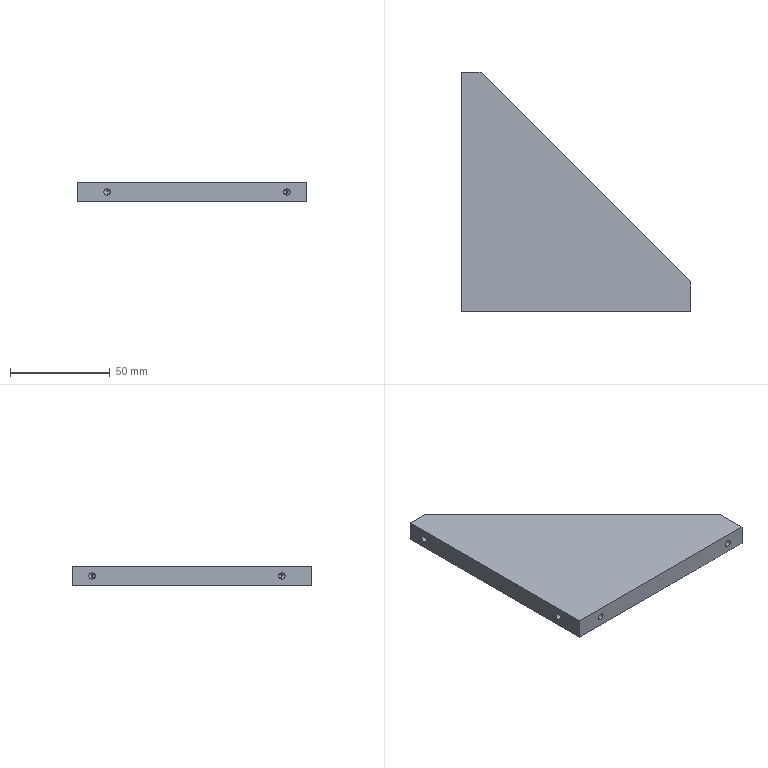Part | SolidWorks | features HoleWzd 4, ICE 4, Fillet 2, ExtruThin 1, Gusset 1 | 1 solid | 23 faces | box 115 x 120 x 10 mm | volume 82518 mm3 | cylinder 8 | cone 8 | plane 7 | commonest cylinder face diameters 3.3 x8
STEP:
#1=CARTESIAN_POINT('',(10.1,110.,28.35));
#2=VERTEX_POINT('',#1);
#3=CARTESIAN_POINT('',(10.1,110.,31.65));
#4=VERTEX_POINT('',#3);
#5=CARTESIAN_POINT('',(10.1,110.,30.));
#6=DIRECTION('',(-1.,0.,0.));
#7=DIRECTION('',(0.,0.,1.));
#8=AXIS2_PLACEMENT_3D('',#5,#6,#7);
#9=CIRCLE('',#8,1.65);
#10=EDGE_CURVE('',#2,#4,#9,.T.);
#11=ORIENTED_EDGE('',*,*,#10,.F.);
#12=CARTESIAN_POINT('',(0.,110.,28.35));
#13=VERTEX_POINT('',#12);
#14=CARTESIAN_POINT('',(0.,110.,28.35));
#15=DIRECTION('',(-1.,0.,0.));
#16=VECTOR('',#15,1000.);
#17=LINE('',#14,#16);
#18=EDGE_CURVE('',#2,#13,#17,.T.);
#19=ORIENTED_EDGE('',*,*,#18,.T.);
#20=CARTESIAN_POINT('',(0.,110.,31.65));
#21=VERTEX_POINT('',#20);
#22=CARTESIAN_POINT('',(0.,110.,30.));
#23=DIRECTION('',(-1.,0.,0.));
#24=DIRECTION('',(0.,0.,1.));
#25=AXIS2_PLACEMENT_3D('',#22,#23,#24);
#26=CIRCLE('',#25,1.65);
#27=EDGE_CURVE('',#13,#21,#26,.T.);
#28=ORIENTED_EDGE('',*,*,#27,.T.);
#29=CARTESIAN_POINT('',(0.,110.,31.65));
#30=DIRECTION('',(-1.,0.,0.));
#31=VECTOR('',#30,1000.);
#32=LINE('',#29,#31);
#33=EDGE_CURVE('',#4,#21,#32,.T.);
#34=ORIENTED_EDGE('',*,*,#33,.F.);
#35=EDGE_LOOP('',(#11,#19,#28,#34));
#36=FACE_OUTER_BOUND('',#35,.T.);
#37=CARTESIAN_POINT('',(0.,110.,30.));
#38=DIRECTION('',(-1.,0.,0.));
#39=DIRECTION('',(0.,0.,1.));
#40=AXIS2_PLACEMENT_3D('',#37,#38,#39);
#41=CYLINDRICAL_SURFACE('',#40,1.65);
#42=ADVANCED_FACE('',(#36),#41,.F.);
#43=CARTESIAN_POINT('',(11.091,110.,30.));
#44=VERTEX_POINT('',#43);
#45=CARTESIAN_POINT('',(10.1,110.,31.65));
#46=DIRECTION('',(-0.515,0.,0.8572));
#47=VECTOR('',#46,1000.);
#48=LINE('',#45,#47);
#49=EDGE_CURVE('',#44,#4,#48,.T.);
#50=ORIENTED_EDGE('',*,*,#49,.F.);
#51=CARTESIAN_POINT('',(10.1,110.,28.35));
#52=DIRECTION('',(-0.515,0.,-0.8572));
#53=VECTOR('',#52,1000.);
#54=LINE('',#51,#53);
#55=EDGE_CURVE('',#44,#2,#54,.T.);
#56=ORIENTED_EDGE('',*,*,#55,.T.);
#57=ORIENTED_EDGE('',*,*,#10,.T.);
#58=EDGE_LOOP('',(#50,#56,#57));
#59=FACE_OUTER_BOUND('',#58,.T.);
#60=CARTESIAN_POINT('',(10.1,110.,30.));
#61=DIRECTION('',(-1.,0.,0.));
#62=DIRECTION('',(0.,0.,1.));
#63=AXIS2_PLACEMENT_3D('',#60,#61,#62);
#64=CONICAL_SURFACE('',#63,1.65,1.03);
#65=ADVANCED_FACE('',(#59),#64,.F.);
#66=CARTESIAN_POINT('',(10.1,15.,28.35));
#67=VERTEX_POINT('',#66);
#68=CARTESIAN_POINT('',(10.1,15.,31.65));
#69=VERTEX_POINT('',#68);
#70=CARTESIAN_POINT('',(10.1,15.,30.));
#71=DIRECTION('',(-1.,0.,0.));
#72=DIRECTION('',(0.,0.,1.));
#73=AXIS2_PLACEMENT_3D('',#70,#71,#72);
#74=CIRCLE('',#73,1.65);
#75=EDGE_CURVE('',#67,#69,#74,.T.);
#76=ORIENTED_EDGE('',*,*,#75,.F.);
#77=CARTESIAN_POINT('',(0.,15.,28.35));
#78=VERTEX_POINT('',#77);
#79=CARTESIAN_POINT('',(0.,15.,28.35));
#80=DIRECTION('',(-1.,0.,0.));
#81=VECTOR('',#80,1000.);
#82=LINE('',#79,#81);
#83=EDGE_CURVE('',#67,#78,#82,.T.);
#84=ORIENTED_EDGE('',*,*,#83,.T.);
#85=CARTESIAN_POINT('',(0.,15.,31.65));
#86=VERTEX_POINT('',#85);
#87=CARTESIAN_POINT('',(0.,15.,30.));
#88=DIRECTION('',(-1.,0.,0.));
#89=DIRECTION('',(0.,0.,1.));
#90=AXIS2_PLACEMENT_3D('',#87,#88,#89);
#91=CIRCLE('',#90,1.65);
#92=EDGE_CURVE('',#78,#86,#91,.T.);
#93=ORIENTED_EDGE('',*,*,#92,.T.);
#94=CARTESIAN_POINT('',(0.,15.,31.65));
#95=DIRECTION('',(-1.,0.,0.));
#96=VECTOR('',#95,1000.);
#97=LINE('',#94,#96);
#98=EDGE_CURVE('',#69,#86,#97,.T.);
#99=ORIENTED_EDGE('',*,*,#98,.F.);
#100=EDGE_LOOP('',(#76,#84,#93,#99));
#101=FACE_OUTER_BOUND('',#100,.T.);
#102=CARTESIAN_POINT('',(0.,15.,30.));
#103=DIRECTION('',(-1.,0.,0.));
#104=DIRECTION('',(0.,0.,1.));
#105=AXIS2_PLACEMENT_3D('',#102,#103,#104);
#106=CYLINDRICAL_SURFACE('',#105,1.65);
#107=ADVANCED_FACE('',(#101),#106,.F.);
#108=CARTESIAN_POINT('',(11.091,15.,30.));
#109=VERTEX_POINT('',#108);
#110=CARTESIAN_POINT('',(10.1,15.,31.65));
#111=DIRECTION('',(-0.515,0.,0.8572));
#112=VECTOR('',#111,1000.);
#113=LINE('',#110,#112);
#114=EDGE_CURVE('',#109,#69,#113,.T.);
#115=ORIENTED_EDGE('',*,*,#114,.F.);
#116=CARTESIAN_POINT('',(10.1,15.,28.35));
#117=DIRECTION('',(-0.515,0.,-0.8572));
#118=VECTOR('',#117,1000.);
#119=LINE('',#116,#118);
#120=EDGE_CURVE('',#109,#67,#119,.T.);
#121=ORIENTED_EDGE('',*,*,#120,.T.);
#122=ORIENTED_EDGE('',*,*,#75,.T.);
#123=EDGE_LOOP('',(#115,#121,#122));
#124=FACE_OUTER_BOUND('',#123,.T.);
#125=CARTESIAN_POINT('',(10.1,15.,30.));
#126=DIRECTION('',(-1.,0.,0.));
#127=DIRECTION('',(0.,0.,1.));
#128=AXIS2_PLACEMENT_3D('',#125,#126,#127);
#129=CONICAL_SURFACE('',#128,1.65,1.03);
#130=ADVANCED_FACE('',(#124),#129,.F.);
#131=CARTESIAN_POINT('',(105.,10.1,31.65));
#132=VERTEX_POINT('',#131);
#133=CARTESIAN_POINT('',(105.,10.1,28.35));
#134=VERTEX_POINT('',#133);
#135=CARTESIAN_POINT('',(105.,10.1,30.));
#136=DIRECTION('',(0.,-1.,0.));
#137=DIRECTION('',(0.,0.,-1.));
#138=AXIS2_PLACEMENT_3D('',#135,#136,#137);
#139=CIRCLE('',#138,1.65);
#140=EDGE_CURVE('',#132,#134,#139,.T.);
#141=ORIENTED_EDGE('',*,*,#140,.F.);
#142=CARTESIAN_POINT('',(105.,0.,31.65));
#143=VERTEX_POINT('',#142);
#144=CARTESIAN_POINT('',(105.,0.,31.65));
#145=DIRECTION('',(0.,-1.,0.));
#146=VECTOR('',#145,1000.);
#147=LINE('',#144,#146);
#148=EDGE_CURVE('',#132,#143,#147,.T.);
#149=ORIENTED_EDGE('',*,*,#148,.T.);
#150=CARTESIAN_POINT('',(105.,0.,28.35));
#151=VERTEX_POINT('',#150);
#152=CARTESIAN_POINT('',(105.,0.,30.));
#153=DIRECTION('',(0.,-1.,0.));
#154=DIRECTION('',(0.,0.,-1.));
#155=AXIS2_PLACEMENT_3D('',#152,#153,#154);
#156=CIRCLE('',#155,1.65);
#157=EDGE_CURVE('',#143,#151,#156,.T.);
#158=ORIENTED_EDGE('',*,*,#157,.T.);
#159=CARTESIAN_POINT('',(105.,0.,28.35));
#160=DIRECTION('',(0.,-1.,0.));
#161=VECTOR('',#160,1000.);
#162=LINE('',#159,#161);
#163=EDGE_CURVE('',#134,#151,#162,.T.);
#164=ORIENTED_EDGE('',*,*,#163,.F.);
#165=EDGE_LOOP('',(#141,#149,#158,#164));
#166=FACE_OUTER_BOUND('',#165,.T.);
#167=CARTESIAN_POINT('',(105.,0.,30.));
#168=DIRECTION('',(0.,-1.,0.));
#169=DIRECTION('',(0.,0.,-1.));
#170=AXIS2_PLACEMENT_3D('',#167,#168,#169);
#171=CYLINDRICAL_SURFACE('',#170,1.65);
#172=ADVANCED_FACE('',(#166),#171,.F.);
#173=CARTESIAN_POINT('',(105.,11.091,30.));
#174=VERTEX_POINT('',#173);
#175=CARTESIAN_POINT('',(105.,10.1,28.35));
#176=DIRECTION('',(0.,-0.515,-0.8572));
#177=VECTOR('',#176,1000.);
#178=LINE('',#175,#177);
#179=EDGE_CURVE('',#174,#134,#178,.T.);
#180=ORIENTED_EDGE('',*,*,#179,.F.);
#181=CARTESIAN_POINT('',(105.,10.1,31.65));
#182=DIRECTION('',(0.,-0.515,0.8572));
#183=VECTOR('',#182,1000.);
#184=LINE('',#181,#183);
#185=EDGE_CURVE('',#174,#132,#184,.T.);
#186=ORIENTED_EDGE('',*,*,#185,.T.);
#187=ORIENTED_EDGE('',*,*,#140,.T.);
#188=EDGE_LOOP('',(#180,#186,#187));
#189=FACE_OUTER_BOUND('',#188,.T.);
#190=CARTESIAN_POINT('',(105.,10.1,30.));
#191=DIRECTION('',(0.,-1.,0.));
#192=DIRECTION('',(0.,0.,-1.));
#193=AXIS2_PLACEMENT_3D('',#190,#191,#192);
#194=CONICAL_SURFACE('',#193,1.65,1.03);
#195=ADVANCED_FACE('',(#189),#194,.F.);
#196=CARTESIAN_POINT('',(15.,10.1,31.65));
#197=VERTEX_POINT('',#196);
#198=CARTESIAN_POINT('',(15.,10.1,28.35));
#199=VERTEX_POINT('',#198);
#200=CARTESIAN_POINT('',(15.,10.1,30.));
#201=DIRECTION('',(0.,-1.,0.));
#202=DIRECTION('',(0.,0.,-1.));
#203=AXIS2_PLACEMENT_3D('',#200,#201,#202);
#204=CIRCLE('',#203,1.65);
#205=EDGE_CURVE('',#197,#199,#204,.T.);
#206=ORIENTED_EDGE('',*,*,#205,.F.);
#207=CARTESIAN_POINT('',(15.,0.,31.65));
#208=VERTEX_POINT('',#207);
#209=CARTESIAN_POINT('',(15.,0.,31.65));
#210=DIRECTION('',(0.,-1.,0.));
#211=VECTOR('',#210,1000.);
#212=LINE('',#209,#211);
#213=EDGE_CURVE('',#197,#208,#212,.T.);
#214=ORIENTED_EDGE('',*,*,#213,.T.);
#215=CARTESIAN_POINT('',(15.,0.,28.35));
#216=VERTEX_POINT('',#215);
#217=CARTESIAN_POINT('',(15.,0.,30.));
#218=DIRECTION('',(0.,-1.,0.));
#219=DIRECTION('',(0.,0.,-1.));
#220=AXIS2_PLACEMENT_3D('',#217,#218,#219);
#221=CIRCLE('',#220,1.65);
#222=EDGE_CURVE('',#208,#216,#221,.T.);
#223=ORIENTED_EDGE('',*,*,#222,.T.);
#224=CARTESIAN_POINT('',(15.,0.,28.35));
#225=DIRECTION('',(0.,-1.,0.));
#226=VECTOR('',#225,1000.);
#227=LINE('',#224,#226);
#228=EDGE_CURVE('',#199,#216,#227,.T.);
#229=ORIENTED_EDGE('',*,*,#228,.F.);
#230=EDGE_LOOP('',(#206,#214,#223,#229));
#231=FACE_OUTER_BOUND('',#230,.T.);
#232=CARTESIAN_POINT('',(15.,0.,30.));
#233=DIRECTION('',(0.,-1.,0.));
#234=DIRECTION('',(0.,0.,-1.));
#235=AXIS2_PLACEMENT_3D('',#232,#233,#234);
#236=CYLINDRICAL_SURFACE('',#235,1.65);
#237=ADVANCED_FACE('',(#231),#236,.F.);
#238=CARTESIAN_POINT('',(15.,11.091,30.));
#239=VERTEX_POINT('',#238);
#240=CARTESIAN_POINT('',(15.,10.1,28.35));
#241=DIRECTION('',(0.,-0.515,-0.8572));
#242=VECTOR('',#241,1000.);
#243=LINE('',#240,#242);
#244=EDGE_CURVE('',#239,#199,#243,.T.);
#245=ORIENTED_EDGE('',*,*,#244,.F.);
#246=CARTESIAN_POINT('',(15.,10.1,31.65));
#247=DIRECTION('',(0.,-0.515,0.8572));
#248=VECTOR('',#247,1000.);
#249=LINE('',#246,#248);
#250=EDGE_CURVE('',#239,#197,#249,.T.);
#251=ORIENTED_EDGE('',*,*,#250,.T.);
#252=ORIENTED_EDGE('',*,*,#205,.T.);
#253=EDGE_LOOP('',(#245,#251,#252));
#254=FACE_OUTER_BOUND('',#253,.T.);
#255=CARTESIAN_POINT('',(15.,10.1,30.));
#256=DIRECTION('',(0.,-1.,0.));
#257=DIRECTION('',(0.,0.,-1.));
#258=AXIS2_PLACEMENT_3D('',#255,#256,#257);
#259=CONICAL_SURFACE('',#258,1.65,1.03);
#260=ADVANCED_FACE('',(#254),#259,.F.);
#261=CARTESIAN_POINT('',(0.,120.,35.));
#262=VERTEX_POINT('',#261);
#263=CARTESIAN_POINT('',(10.,120.,35.));
#264=VERTEX_POINT('',#263);
#265=CARTESIAN_POINT('',(0.,120.,35.));
#266=DIRECTION('',(1.,0.,0.));
#267=VECTOR('',#266,1000.);
#268=LINE('',#265,#267);
#269=EDGE_CURVE('',#262,#264,#268,.T.);
#270=ORIENTED_EDGE('',*,*,#269,.T.);
#271=CARTESIAN_POINT('',(10.,120.,25.));
#272=VERTEX_POINT('',#271);
#273=CARTESIAN_POINT('',(10.,120.,25.));
#274=DIRECTION('',(0.,0.,1.));
#275=VECTOR('',#274,1000.);
#276=LINE('',#273,#275);
#277=EDGE_CURVE('',#272,#264,#276,.T.);
#278=ORIENTED_EDGE('',*,*,#277,.F.);
#279=CARTESIAN_POINT('',(0.,120.,25.));
#280=VERTEX_POINT('',#279);
#281=CARTESIAN_POINT('',(0.,120.,25.));
#282=DIRECTION('',(1.,0.,0.));
#283=VECTOR('',#282,1000.);
#284=LINE('',#281,#283);
#285=EDGE_CURVE('',#280,#272,#284,.T.);
#286=ORIENTED_EDGE('',*,*,#285,.F.);
#287=CARTESIAN_POINT('',(0.,120.,25.));
#288=DIRECTION('',(0.,0.,1.));
#289=VECTOR('',#288,1000.);
#290=LINE('',#287,#289);
#291=EDGE_CURVE('',#280,#262,#290,.T.);
#292=ORIENTED_EDGE('',*,*,#291,.T.);
#293=EDGE_LOOP('',(#270,#278,#286,#292));
#294=FACE_OUTER_BOUND('',#293,.T.);
#295=CARTESIAN_POINT('',(0.,120.,25.));
#296=DIRECTION('',(0.,-1.,0.));
#297=DIRECTION('',(0.,0.,-1.));
#298=AXIS2_PLACEMENT_3D('',#295,#296,#297);
#299=PLANE('',#298);
#300=ADVANCED_FACE('',(#294),#299,.F.);
#301=CARTESIAN_POINT('',(115.,15.,35.));
#302=VERTEX_POINT('',#301);
#303=CARTESIAN_POINT('',(10.,120.,35.));
#304=DIRECTION('',(0.7071,-0.7071,0.));
#305=VECTOR('',#304,1000.);
#306=LINE('',#303,#305);
#307=EDGE_CURVE('',#264,#302,#306,.T.);
#308=ORIENTED_EDGE('',*,*,#307,.T.);
#309=CARTESIAN_POINT('',(115.,15.,25.));
#310=VERTEX_POINT('',#309);
#311=CARTESIAN_POINT('',(115.,15.,25.));
#312=DIRECTION('',(0.,0.,1.));
#313=VECTOR('',#312,1000.);
#314=LINE('',#311,#313);
#315=EDGE_CURVE('',#310,#302,#314,.T.);
#316=ORIENTED_EDGE('',*,*,#315,.F.);
#317=CARTESIAN_POINT('',(10.,120.,25.));
#318=DIRECTION('',(0.7071,-0.7071,0.));
#319=VECTOR('',#318,1000.);
#320=LINE('',#317,#319);
#321=EDGE_CURVE('',#272,#310,#320,.T.);
#322=ORIENTED_EDGE('',*,*,#321,.F.);
#323=ORIENTED_EDGE('',*,*,#277,.T.);
#324=EDGE_LOOP('',(#308,#316,#322,#323));
#325=FACE_OUTER_BOUND('',#324,.T.);
#326=CARTESIAN_POINT('',(10.,120.,25.));
#327=DIRECTION('',(-0.7071,-0.7071,0.));
#328=DIRECTION('',(0.7071,-0.7071,0.));
#329=AXIS2_PLACEMENT_3D('',#326,#327,#328);
#330=PLANE('',#329);
#331=ADVANCED_FACE('',(#325),#330,.F.);
#332=CARTESIAN_POINT('',(115.,0.,35.));
#333=VERTEX_POINT('',#332);
#334=CARTESIAN_POINT('',(115.,0.,35.));
#335=DIRECTION('',(0.,-1.,0.));
#336=VECTOR('',#335,1000.);
#337=LINE('',#334,#336);
#338=EDGE_CURVE('',#302,#333,#337,.T.);
#339=ORIENTED_EDGE('',*,*,#338,.T.);
#340=CARTESIAN_POINT('',(115.,0.,25.));
#341=VERTEX_POINT('',#340);
#342=CARTESIAN_POINT('',(115.,0.,25.));
#343=DIRECTION('',(0.,0.,1.));
#344=VECTOR('',#343,1000.);
#345=LINE('',#342,#344);
#346=EDGE_CURVE('',#341,#333,#345,.T.);
#347=ORIENTED_EDGE('',*,*,#346,.F.);
#348=CARTESIAN_POINT('',(115.,0.,25.));
#349=DIRECTION('',(0.,-1.,0.));
#350=VECTOR('',#349,1000.);
#351=LINE('',#348,#350);
#352=EDGE_CURVE('',#310,#341,#351,.T.);
#353=ORIENTED_EDGE('',*,*,#352,.F.);
#354=ORIENTED_EDGE('',*,*,#315,.T.);
#355=EDGE_LOOP('',(#339,#347,#353,#354));
#356=FACE_OUTER_BOUND('',#355,.T.);
#357=CARTESIAN_POINT('',(115.,0.,25.));
#358=DIRECTION('',(-1.,0.,0.));
#359=DIRECTION('',(0.,0.,1.));
#360=AXIS2_PLACEMENT_3D('',#357,#358,#359);
#361=PLANE('',#360);
#362=ADVANCED_FACE('',(#356),#361,.F.);
#363=CARTESIAN_POINT('',(105.,0.,30.));
#364=DIRECTION('',(0.,-1.,0.));
#365=DIRECTION('',(0.,0.,-1.));
#366=AXIS2_PLACEMENT_3D('',#363,#364,#365);
#367=CIRCLE('',#366,1.65);
#368=EDGE_CURVE('',#151,#143,#367,.T.);
#369=ORIENTED_EDGE('',*,*,#368,.F.);
#370=ORIENTED_EDGE('',*,*,#157,.F.);
#371=EDGE_LOOP('',(#369,#370));
#372=FACE_BOUND('',#371,.T.);
#373=CARTESIAN_POINT('',(15.,0.,30.));
#374=DIRECTION('',(0.,-1.,0.));
#375=DIRECTION('',(0.,0.,-1.));
#376=AXIS2_PLACEMENT_3D('',#373,#374,#375);
#377=CIRCLE('',#376,1.65);
#378=EDGE_CURVE('',#216,#208,#377,.T.);
#379=ORIENTED_EDGE('',*,*,#378,.F.);
#380=ORIENTED_EDGE('',*,*,#222,.F.);
#381=EDGE_LOOP('',(#379,#380));
#382=FACE_BOUND('',#381,.T.);
#383=CARTESIAN_POINT('',(0.,0.,35.));
#384=VERTEX_POINT('',#383);
#385=CARTESIAN_POINT('',(0.,0.,35.));
#386=DIRECTION('',(-1.,0.,0.));
#387=VECTOR('',#386,1000.);
#388=LINE('',#385,#387);
#389=EDGE_CURVE('',#333,#384,#388,.T.);
#390=ORIENTED_EDGE('',*,*,#389,.T.);
#391=CARTESIAN_POINT('',(0.,0.,25.));
#392=VERTEX_POINT('',#391);
#393=CARTESIAN_POINT('',(0.,0.,25.));
#394=DIRECTION('',(0.,0.,1.));
#395=VECTOR('',#394,1000.);
#396=LINE('',#393,#395);
#397=EDGE_CURVE('',#392,#384,#396,.T.);
#398=ORIENTED_EDGE('',*,*,#397,.F.);
#399=CARTESIAN_POINT('',(0.,0.,25.));
#400=DIRECTION('',(-1.,0.,0.));
#401=VECTOR('',#400,1000.);
#402=LINE('',#399,#401);
#403=EDGE_CURVE('',#341,#392,#402,.T.);
#404=ORIENTED_EDGE('',*,*,#403,.F.);
#405=ORIENTED_EDGE('',*,*,#346,.T.);
#406=EDGE_LOOP('',(#390,#398,#404,#405));
#407=FACE_OUTER_BOUND('',#406,.T.);
#408=CARTESIAN_POINT('',(0.,0.,25.));
#409=DIRECTION('',(0.,1.,0.));
#410=DIRECTION('',(0.,0.,1.));
#411=AXIS2_PLACEMENT_3D('',#408,#409,#410);
#412=PLANE('',#411);
#413=ADVANCED_FACE('',(#372,#382,#407),#412,.F.);
#414=CARTESIAN_POINT('',(0.,110.,30.));
#415=DIRECTION('',(-1.,0.,0.));
#416=DIRECTION('',(0.,0.,1.));
#417=AXIS2_PLACEMENT_3D('',#414,#415,#416);
#418=CIRCLE('',#417,1.65);
#419=EDGE_CURVE('',#21,#13,#418,.T.);
#420=ORIENTED_EDGE('',*,*,#419,.F.);
#421=ORIENTED_EDGE('',*,*,#27,.F.);
#422=EDGE_LOOP('',(#420,#421));
#423=FACE_BOUND('',#422,.T.);
#424=CARTESIAN_POINT('',(0.,15.,30.));
#425=DIRECTION('',(-1.,0.,0.));
#426=DIRECTION('',(0.,0.,1.));
#427=AXIS2_PLACEMENT_3D('',#424,#425,#426);
#428=CIRCLE('',#427,1.65);
#429=EDGE_CURVE('',#86,#78,#428,.T.);
#430=ORIENTED_EDGE('',*,*,#429,.F.);
#431=ORIENTED_EDGE('',*,*,#92,.F.);
#432=EDGE_LOOP('',(#430,#431));
#433=FACE_BOUND('',#432,.T.);
#434=CARTESIAN_POINT('',(0.,0.,35.));
#435=DIRECTION('',(0.,1.,0.));
#436=VECTOR('',#435,1000.);
#437=LINE('',#434,#436);
#438=EDGE_CURVE('',#384,#262,#437,.T.);
#439=ORIENTED_EDGE('',*,*,#438,.T.);
#440=ORIENTED_EDGE('',*,*,#291,.F.);
#441=CARTESIAN_POINT('',(0.,0.,25.));
#442=DIRECTION('',(0.,1.,0.));
#443=VECTOR('',#442,1000.);
#444=LINE('',#441,#443);
#445=EDGE_CURVE('',#392,#280,#444,.T.);
#446=ORIENTED_EDGE('',*,*,#445,.F.);
#447=ORIENTED_EDGE('',*,*,#397,.T.);
#448=EDGE_LOOP('',(#439,#440,#446,#447));
#449=FACE_OUTER_BOUND('',#448,.T.);
#450=CARTESIAN_POINT('',(0.,0.,25.));
#451=DIRECTION('',(1.,0.,0.));
#452=DIRECTION('',(0.,1.,0.));
#453=AXIS2_PLACEMENT_3D('',#450,#451,#452);
#454=PLANE('',#453);
#455=ADVANCED_FACE('',(#423,#433,#449),#454,.F.);
#456=ORIENTED_EDGE('',*,*,#285,.T.);
#457=ORIENTED_EDGE('',*,*,#321,.T.);
#458=ORIENTED_EDGE('',*,*,#352,.T.);
#459=ORIENTED_EDGE('',*,*,#403,.T.);
#460=ORIENTED_EDGE('',*,*,#445,.T.);
#461=EDGE_LOOP('',(#456,#457,#458,#459,#460));
#462=FACE_OUTER_BOUND('',#461,.T.);
#463=CARTESIAN_POINT('',(0.,0.,25.));
#464=DIRECTION('',(0.,0.,1.));
#465=DIRECTION('',(1.,0.,0.));
#466=AXIS2_PLACEMENT_3D('',#463,#464,#465);
#467=PLANE('',#466);
#468=ADVANCED_FACE('',(#462),#467,.F.);
#469=ORIENTED_EDGE('',*,*,#269,.F.);
#470=ORIENTED_EDGE('',*,*,#438,.F.);
#471=ORIENTED_EDGE('',*,*,#389,.F.);
#472=ORIENTED_EDGE('',*,*,#338,.F.);
#473=ORIENTED_EDGE('',*,*,#307,.F.);
#474=EDGE_LOOP('',(#469,#470,#471,#472,#473));
#475=FACE_OUTER_BOUND('',#474,.T.);
#476=CARTESIAN_POINT('',(0.,0.,35.));
#477=DIRECTION('',(0.,0.,1.));
#478=DIRECTION('',(1.,0.,0.));
#479=AXIS2_PLACEMENT_3D('',#476,#477,#478);
#480=PLANE('',#479);
#481=ADVANCED_FACE('',(#475),#480,.T.);
#482=ORIENTED_EDGE('',*,*,#250,.F.);
#483=ORIENTED_EDGE('',*,*,#244,.T.);
#484=CARTESIAN_POINT('',(15.,10.1,30.));
#485=DIRECTION('',(0.,-1.,0.));
#486=DIRECTION('',(0.,0.,-1.));
#487=AXIS2_PLACEMENT_3D('',#484,#485,#486);
#488=CIRCLE('',#487,1.65);
#489=EDGE_CURVE('',#199,#197,#488,.T.);
#490=ORIENTED_EDGE('',*,*,#489,.T.);
#491=EDGE_LOOP('',(#482,#483,#490));
#492=FACE_OUTER_BOUND('',#491,.T.);
#493=CARTESIAN_POINT('',(15.,10.1,30.));
#494=DIRECTION('',(0.,-1.,0.));
#495=DIRECTION('',(0.,0.,-1.));
#496=AXIS2_PLACEMENT_3D('',#493,#494,#495);
#497=CONICAL_SURFACE('',#496,1.65,1.03);
#498=ADVANCED_FACE('',(#492),#497,.F.);
#499=ORIENTED_EDGE('',*,*,#213,.F.);
#500=ORIENTED_EDGE('',*,*,#489,.F.);
#501=ORIENTED_EDGE('',*,*,#228,.T.);
#502=ORIENTED_EDGE('',*,*,#378,.T.);
#503=EDGE_LOOP('',(#499,#500,#501,#502));
#504=FACE_OUTER_BOUND('',#503,.T.);
#505=CARTESIAN_POINT('',(15.,0.,30.));
#506=DIRECTION('',(0.,-1.,0.));
#507=DIRECTION('',(0.,0.,-1.));
#508=AXIS2_PLACEMENT_3D('',#505,#506,#507);
#509=CYLINDRICAL_SURFACE('',#508,1.65);
#510=ADVANCED_FACE('',(#504),#509,.F.);
#511=ORIENTED_EDGE('',*,*,#185,.F.);
#512=ORIENTED_EDGE('',*,*,#179,.T.);
#513=CARTESIAN_POINT('',(105.,10.1,30.));
#514=DIRECTION('',(0.,-1.,0.));
#515=DIRECTION('',(0.,0.,-1.));
#516=AXIS2_PLACEMENT_3D('',#513,#514,#515);
#517=CIRCLE('',#516,1.65);
#518=EDGE_CURVE('',#134,#132,#517,.T.);
#519=ORIENTED_EDGE('',*,*,#518,.T.);
#520=EDGE_LOOP('',(#511,#512,#519));
#521=FACE_OUTER_BOUND('',#520,.T.);
#522=CARTESIAN_POINT('',(105.,10.1,30.));
#523=DIRECTION('',(0.,-1.,0.));
#524=DIRECTION('',(0.,0.,-1.));
#525=AXIS2_PLACEMENT_3D('',#522,#523,#524);
#526=CONICAL_SURFACE('',#525,1.65,1.03);
#527=ADVANCED_FACE('',(#521),#526,.F.);
#528=ORIENTED_EDGE('',*,*,#148,.F.);
#529=ORIENTED_EDGE('',*,*,#518,.F.);
#530=ORIENTED_EDGE('',*,*,#163,.T.);
#531=ORIENTED_EDGE('',*,*,#368,.T.);
#532=EDGE_LOOP('',(#528,#529,#530,#531));
#533=FACE_OUTER_BOUND('',#532,.T.);
#534=CARTESIAN_POINT('',(105.,0.,30.));
#535=DIRECTION('',(0.,-1.,0.));
#536=DIRECTION('',(0.,0.,-1.));
#537=AXIS2_PLACEMENT_3D('',#534,#535,#536);
#538=CYLINDRICAL_SURFACE('',#537,1.65);
#539=ADVANCED_FACE('',(#533),#538,.F.);
#540=ORIENTED_EDGE('',*,*,#120,.F.);
#541=ORIENTED_EDGE('',*,*,#114,.T.);
#542=CARTESIAN_POINT('',(10.1,15.,30.));
#543=DIRECTION('',(-1.,0.,0.));
#544=DIRECTION('',(0.,0.,1.));
#545=AXIS2_PLACEMENT_3D('',#542,#543,#544);
#546=CIRCLE('',#545,1.65);
#547=EDGE_CURVE('',#69,#67,#546,.T.);
#548=ORIENTED_EDGE('',*,*,#547,.T.);
#549=EDGE_LOOP('',(#540,#541,#548));
#550=FACE_OUTER_BOUND('',#549,.T.);
#551=CARTESIAN_POINT('',(10.1,15.,30.));
#552=DIRECTION('',(-1.,0.,0.));
#553=DIRECTION('',(0.,0.,1.));
#554=AXIS2_PLACEMENT_3D('',#551,#552,#553);
#555=CONICAL_SURFACE('',#554,1.65,1.03);
#556=ADVANCED_FACE('',(#550),#555,.F.);
#557=ORIENTED_EDGE('',*,*,#83,.F.);
#558=ORIENTED_EDGE('',*,*,#547,.F.);
#559=ORIENTED_EDGE('',*,*,#98,.T.);
#560=ORIENTED_EDGE('',*,*,#429,.T.);
#561=EDGE_LOOP('',(#557,#558,#559,#560));
#562=FACE_OUTER_BOUND('',#561,.T.);
#563=CARTESIAN_POINT('',(0.,15.,30.));
#564=DIRECTION('',(-1.,0.,0.));
#565=DIRECTION('',(0.,0.,1.));
#566=AXIS2_PLACEMENT_3D('',#563,#564,#565);
#567=CYLINDRICAL_SURFACE('',#566,1.65);
#568=ADVANCED_FACE('',(#562),#567,.F.);
#569=ORIENTED_EDGE('',*,*,#55,.F.);
#570=ORIENTED_EDGE('',*,*,#49,.T.);
#571=CARTESIAN_POINT('',(10.1,110.,30.));
#572=DIRECTION('',(-1.,0.,0.));
#573=DIRECTION('',(0.,0.,1.));
#574=AXIS2_PLACEMENT_3D('',#571,#572,#573);
#575=CIRCLE('',#574,1.65);
#576=EDGE_CURVE('',#4,#2,#575,.T.);
#577=ORIENTED_EDGE('',*,*,#576,.T.);
#578=EDGE_LOOP('',(#569,#570,#577));
#579=FACE_OUTER_BOUND('',#578,.T.);
#580=CARTESIAN_POINT('',(10.1,110.,30.));
#581=DIRECTION('',(-1.,0.,0.));
#582=DIRECTION('',(0.,0.,1.));
#583=AXIS2_PLACEMENT_3D('',#580,#581,#582);
#584=CONICAL_SURFACE('',#583,1.65,1.03);
#585=ADVANCED_FACE('',(#579),#584,.F.);
#586=ORIENTED_EDGE('',*,*,#18,.F.);
#587=ORIENTED_EDGE('',*,*,#576,.F.);
#588=ORIENTED_EDGE('',*,*,#33,.T.);
#589=ORIENTED_EDGE('',*,*,#419,.T.);
#590=EDGE_LOOP('',(#586,#587,#588,#589));
#591=FACE_OUTER_BOUND('',#590,.T.);
#592=CARTESIAN_POINT('',(0.,110.,30.));
#593=DIRECTION('',(-1.,0.,0.));
#594=DIRECTION('',(0.,0.,1.));
#595=AXIS2_PLACEMENT_3D('',#592,#593,#594);
#596=CYLINDRICAL_SURFACE('',#595,1.65);
#597=ADVANCED_FACE('',(#591),#596,.F.);
#598=CLOSED_SHELL('',(#42,#65,#107,#130,#172,#195,#237,#260,#300,#331,#362,#413,#455,#468,#481,#498,#510,#527,#539,#556,#568,#585,#597));
#599=MANIFOLD_SOLID_BREP('',#598);
#600=CARTESIAN_POINT('',(0.,0.,0.));
#601=DIRECTION('',(0.,0.,1.));
#602=DIRECTION('',(1.,0.,0.));
#603=AXIS2_PLACEMENT_3D('',#600,#601,#602);
#604=(LENGTH_UNIT()NAMED_UNIT(*)SI_UNIT(.MILLI.,.METRE.));
#605=UNCERTAINTY_MEASURE_WITH_UNIT(LENGTH_MEASURE(0.00001),#604,'','');
#606=(NAMED_UNIT(*)PLANE_ANGLE_UNIT()SI_UNIT($,.RADIAN.));
#607=(NAMED_UNIT(*)SI_UNIT($,.STERADIAN.)SOLID_ANGLE_UNIT());
#608=(GEOMETRIC_REPRESENTATION_CONTEXT(3)GLOBAL_UNCERTAINTY_ASSIGNED_CONTEXT((#605))GLOBAL_UNIT_ASSIGNED_CONTEXT((#604,#606,#607))REPRESENTATION_CONTEXT('',''));
#609=ADVANCED_BREP_SHAPE_REPRESENTATION('',(#599,#603),#608);